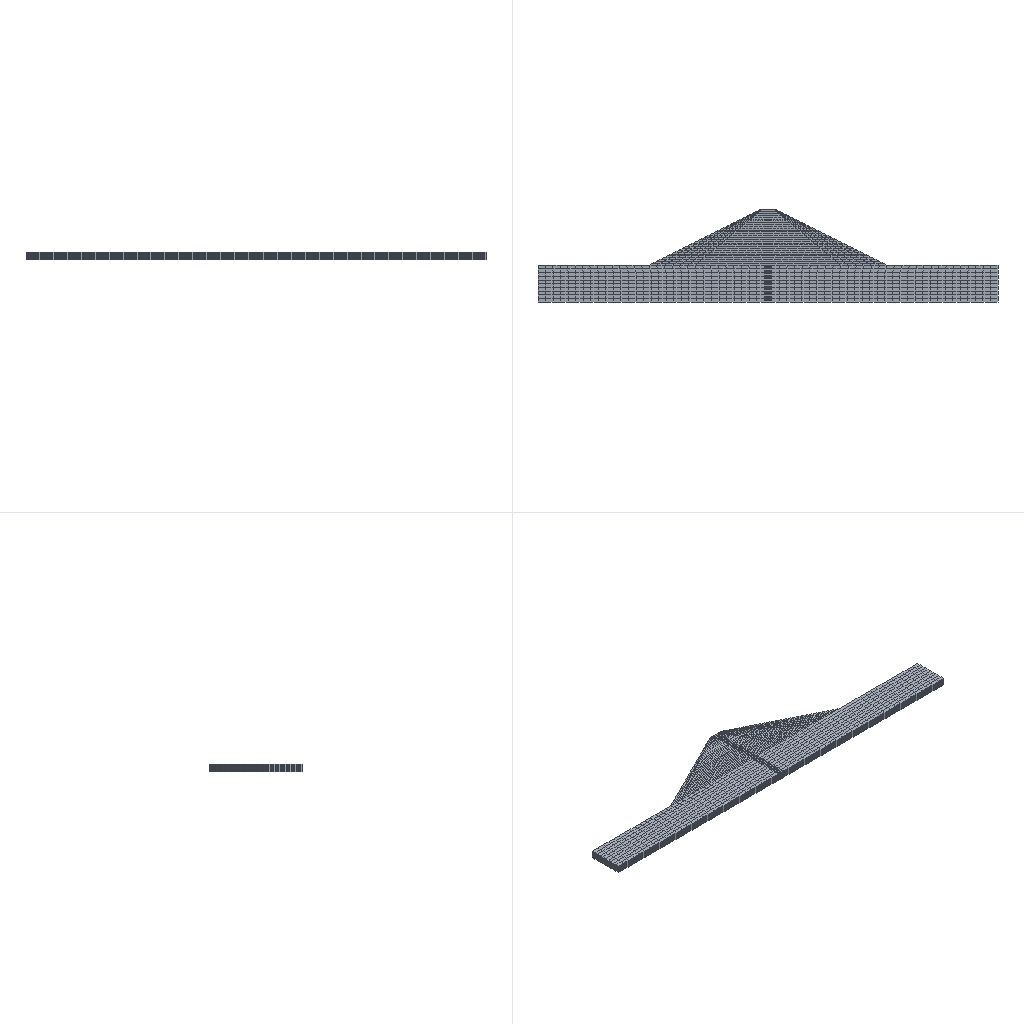Simulation study | abaqus
Set-up summary:
category,name,step,type,value,unit,region
solver,abaqus
solver,version,,,Abaqus/Standard 2020
units,not stated in the deck,,not stated
analysis,deck,,soils,soils
load_step,shenliu,shenliu,soils
load_step,requested,,,1
mesh,nodes,,,23364
mesh,elements,,,19432
element_type,C3D8P,,solid,19432
load,load commands in deck,,count,300
bc,support commands in deck,,count,311
material,BAJI,,in results
material,BATI,,in results
material,QIANG,,in results
check,setup vs results,,match,"per instance, exact: element labels, types and connectivity; labels of the nodes the elements use; coordinates of those nodes at SINGLE_PRECISION in 1 of 2 instance(s)"
Abaqus input file, long lists of numbers shortened:
*Heading
** Job name: Job-3 Model name: 3cm14mML300-OH-shenliu
** Generated by: Abaqus/CAE 2020
*Preprint, echo=NO, model=NO, history=NO, contact=NO
**
** PARTS
**
*Part, name=ba
*End Part
**
*Part, name=qiang
*End Part
**
**
** ASSEMBLY
**
*Assembly, name=Assembly
**
*Instance, name=ba-1, part=ba
*Node
      1,   62.235,         23.5,  0.9
      2,   62.235,         23.5,           0.
** (22570 more lines like these left out)
*Element, type=C3D8P
 1,     1,   169,  2647,   180,   195,  2677, 12325,  2665
 2,   169,   170,  2648,  2647,  2677,  2678, 12326, 12325
** (19078 more lines like these left out)
*Nset, nset=Set-1
     1,     2,     3,     4,     5,     6,     7,     8,     9,    10,    11,    12,    13,    14,    15,    16
    17,    18,    19,    20,    21,    22,    23,    24,    25,    26,    27,    28,    29,    30,    31,    32
** (894 more lines like these left out)
*Elset, elset=Set-1
     1,     2,     3,     4,     5,     6,     7,     8,     9,    10,    11,    12,    13,    14,    15,    16
    17,    18,    19,    20,    21,    22,    23,    24,    25,    26,    27,    28,    29,    30,    31,    32
** (748 more lines like these left out)
*Nset, nset=Set-2
    31,    32,    33,    34,    35,    36,    37,    38,    39,    40,    41,    42,    43,    44,    45,    52
    53,    54,    55,    58,    59,    62,    63,    65,    68,    69,    71,    74,    75,    77,    95,    96
** (543 more lines like these left out)
*Elset, elset=Set-2, generate
  9949,  17028,      1
** Section: bati
*Solid Section, elset=Set-1, material=bati
,
** Section: baji
*Solid Section, elset=Set-2, material=baji
,
*End Instance
**
*Instance, name=qiang-1, part=qiang
      62.235,           8.,           0.
*Node
      1,           0.,         15.5,   1.2
      2, 0.03,         15.5,   1.2
** (790 more lines like these left out)
*Element, type=C3D8P
 1,  84, 111, 110,  33,   1,   2,   3,   4
 2,  83, 112, 109,  34,  84, 111, 110,  33
** (350 more lines like these left out)
*Nset, nset=Set-1, generate
   1,  792,    1
*Elset, elset=Set-1, generate
   1,  352,    1
** Section: qiang
*Solid Section, elset=Set-1, material=qiang
,
*End Instance
**
*Nset, nset=Set-1, instance=ba-1
    31,    32,    33,    34,    35,    36,    37,    38,    39,    40,    41,    42,    43,    44,    45,    52
    53,    54,    55,    58,    59,    62,    63,    65,    68,    69,    71,    74,    75,    77,    95,    96
** (543 more lines like these left out)
*Elset, elset=Set-1, instance=ba-1, generate
  9949,  17028,      1
*Nset, nset=Set-2, instance=ba-1
   131,   132,   133,   134,   135,   136,   138,   139,   143,   144,   145,   146,   147,   148,   154,   155
   156,   158,   162,   163,   165,   166,   167,   168,  1801,  1802,  1803,  1804,  1805,  1806,  1807,  1808
** (14 more lines like these left out)
*Elset, elset=Set-2, instance=ba-1
 10961, 10962, 10963, 10964, 10965, 10966, 10967, 10968, 11085, 11086, 11087, 11088, 11321, 11322, 11323, 11324
 11325, 11326, 11327, 11328, 11525, 11526, 11527, 11528, 11529, 11530, 11531, 11532, 11533, 11534, 11535, 11536
** (11 more lines like these left out)
*Nset, nset=Set-3, instance=ba-1
    97,    98,   101,   102,   104,   106,   108,   109,   112,   115,   116,   117,   121,   122,   124,   125
   151,   152,   153,   154,   155,   156,   157,   158,   159,   160,   161,   162,   163,   164,   165,   167
** (48 more lines like these left out)
*Elset, elset=Set-3, instance=ba-1
  9963,  9964,  9979,  9980,  9995,  9996, 10011, 10012, 10041, 10042, 10043, 10044, 10073, 10074, 10075, 10076
 10105, 10106, 10107, 10108, 10137, 10138, 10139, 10140, 10148, 10156, 10185, 10186, 10187, 10188, 10301, 10302
** (43 more lines like these left out)
*Nset, nset=Set-4, instance=ba-1
     2,     3,     6,     7,    13,    15,    16,    18,    20,    22,    27,    28,    29,    30,    32,    33
    37,    39,    41,    44,    45,    46,    47,    60,    61,    62,    63,    64,    65,    67,    69,    72
** (255 more lines like these left out)
*Nset, nset=Set-4, instance=qiang-1
   9,  10,  11,  12,  17,  18,  19,  20,  21,  22,  23,  24,  26,  27,  31,  32
 145, 146, 147, 148, 149, 150, 151, 152, 153, 154, 155, 156, 157, 158, 159, 160
** (7 more lines like these left out)
*Elset, elset=Set-4, instance=ba-1
     4,     8,    12,    16,    20,    24,    28,    32,    36,    40,    44,    48,    73,    77,    81,    85
    89,    93,    97,   101,   105,   109,   113,   117,   121,   125,   129,   133,   137,   141,   145,   149
** (237 more lines like these left out)
*Elset, elset=Set-4, instance=qiang-1
  30,  33,  36,  39,  42,  45,  48,  51,  54,  57,  60,  63,  66,  69,  72,  75
  78,  81,  84,  87,  90,  93,  96,  99, 102, 105, 108, 114, 117, 120, 121, 122
** (2 more lines like these left out)
*Nset, nset=Set-6, instance=ba-1
     5,     6,    12,    19,    20,    21,    22,    24,    26,    28,    30,    31,    32,    33,    34,    35
    36,    37,    38,    39,    40,    41,    42,    43,    44,    45,    47,    52,    53,    54,    55,    56
** (599 more lines like these left out)
*Nset, nset=Set-6, instance=qiang-1
  13,  14,  15,  16,  17,  18,  19,  20,  21,  22,  23,  24,  25,  26,  27,  28
  29,  30,  31,  32, 205, 206, 207, 208, 213, 214, 215, 216, 217, 218, 219, 220
** (5 more lines like these left out)
*Elset, elset=Set-6, instance=ba-1
    33,    34,    35,    36,    65,    69,   141,   142,   143,   144,   201,   202,   203,   204,   261,   262
   263,   264,   265,   280,   295,   310,   325,   340,   355,   370,   385,   400,   415,   430,   445,   460
** (491 more lines like these left out)
*Elset, elset=Set-6, instance=qiang-1
 111, 118, 119, 120, 121, 122, 123, 126, 129, 132, 135, 138, 141, 142, 143, 144
 145, 146, 147, 148, 149, 150, 151, 152, 153, 154, 155, 156, 157, 158, 159, 160
** (2 more lines like these left out)
*Nset, nset=Set-7, instance=ba-1, generate
     1,  22572,      1
*Nset, nset=Set-7, instance=qiang-1, generate
   1,  792,    1
*Elset, elset=Set-7, instance=ba-1, generate
     1,  19080,      1
*Elset, elset=Set-7, instance=qiang-1, generate
   1,  352,    1
*Nset, nset=Set-8, instance=ba-1
    31,    32,    33,    34,    35,    36,    37,    38,    39,    40,    41,    42,    43,    44,    45,    52
    53,    54,    55,    58,    59,    62,    63,    65,    68,    69,    71,    74,    75,    77,    95,    96
** (543 more lines like these left out)
*Elset, elset=Set-8, instance=ba-1, generate
  9949,  17028,      1
*Nset, nset=Set-9, instance=ba-1
    31,    32,    33,    34,    35,    36,    37,    38,    39,    40,    41,    42,    43,    44,    45,    52
    53,    54,    55,    58,    59,    62,    63,    65,    68,    69,    71,    74,    75,    77,    95,    96
** (543 more lines like these left out)
*Elset, elset=Set-9, instance=ba-1, generate
  9949,  17028,      1
*Nset, nset=Set-10, instance=ba-1
    31,    32,    33,    34,    35,    36,    37,    38,    39,    40,    41,    42,    43,    44,    45,    52
    53,    54,    55,    58,    59,    62,    63,    65,    68,    69,    71,    74,    75,    77,    95,    96
** (543 more lines like these left out)
*Elset, elset=Set-10, instance=ba-1, generate
  9949,  17028,      1
*Nset, nset=Set-12, instance=ba-1
   19,   20,   24,   28,   40,   41,   43,   45,  247,  248,  249,  314,  352,  353,  354,  650
  651,  652,  667,  668,  669,  670,  671,  672,  673,  674,  675,  676,  677,  678,  679,  680
** (18 more lines like these left out)
*Elset, elset=Set-12, instance=ba-1
 1365, 1366, 1367, 1368, 1425, 1426, 1427, 1428, 1485, 1486, 1487, 1488, 1545, 1546, 1547, 1548
 1605, 1606, 1607, 1608, 1665, 1666, 1667, 1668, 1725, 1726, 1727, 1728, 1785, 1786, 1787, 1788
** (15 more lines like these left out)
*Nset, nset=Set-15, instance=ba-1
    31,    32,    33,    34,    35,    36,    37,    38,    39,    40,    41,    42,    43,    44,    45,    52
    53,    54,    55,    58,    59,    62,    63,    65,    68,    69,    71,    74,    75,    77,    95,    96
** (543 more lines like these left out)
*Elset, elset=Set-15, instance=ba-1, generate
  9949,  17028,      1
*Nset, nset=Set-21, instance=ba-1
    31,    32,    33,    34,    35,    36,    37,    38,    39,    40,    41,    42,    43,    44,    45,    52
    53,    54,    55,    58,    59,    62,    63,    65,    68,    69,    71,    74,    75,    77,    95,    96
** (543 more lines like these left out)
*Elset, elset=Set-21, instance=ba-1, generate
  9949,  17028,      1
*Nset, nset=Set-22, instance=ba-1
    31,    32,    33,    34,    35,    36,    37,    38,    39,    40,    41,    42,    43,    44,    45,    52
    53,    54,    55,    58,    59,    62,    63,    65,    68,    69,    71,    74,    75,    77,    95,    96
** (543 more lines like these left out)
*Elset, elset=Set-22, instance=ba-1, generate
  9949,  17028,      1
*Nset, nset=Set-23, instance=ba-1, generate
     1,  22572,      1
*Nset, nset=Set-23, instance=qiang-1, generate
   1,  792,    1
*Elset, elset=Set-23, instance=ba-1, generate
     1,  19080,      1
*Elset, elset=Set-23, instance=qiang-1, generate
   1,  352,    1
*Nset, nset=Set-33, instance=ba-1
    56,    57,    58,    59,    61,    63,    82,    83,    85,    93,    94,   150,  1009,  1038,  1039,  1040
  1041,  1042,  1043,  1044,  1045,  1046,  1047,  1048,  1049,  1050,  1051,  1052,  1053,  1054,  1055,  1056
** (20 more lines like these left out)
*Elset, elset=Set-33, instance=ba-1
  5623,  5638,  5653,  5668,  5683,  5698,  5713,  5728,  5743,  5758,  5773,  5788,  5803,  5818,  5833,  5848
  5863,  5878,  5893,  5908,  5923,  5938,  5953,  5968,  5983,  5998,  6013,  6028,  6043,  6058,  6073,  6088
** (17 more lines like these left out)
*Nset, nset=Set-34, instance=ba-1, generate
     1,  22572,      1
*Nset, nset=Set-34, instance=qiang-1, generate
   1,  792,    1
*Elset, elset=Set-34, instance=ba-1, generate
     1,  19080,      1
*Elset, elset=Set-34, instance=qiang-1, generate
   1,  352,    1
*Nset, nset=Set-35, instance=ba-1
    56,    57,    58,    59,    61,    63,    82,    83,    85,    93,    94,    97,    98,   101,   102,   104
   106,   108,   109,   112,   115,   116,   117,   121,   122,   124,   125,   143,   144,   145,   146,   147
** (86 more lines like these left out)
*Elset, elset=Set-35, instance=ba-1
  5623,  5638,  5653,  5668,  5683,  5698,  5713,  5728,  5743,  5758,  5773,  5788,  5803,  5818,  5833,  5848
  5863,  5878,  5893,  5908,  5923,  5938,  5953,  5968,  5983,  5998,  6013,  6028,  6043,  6058,  6073,  6088
** (76 more lines like these left out)
*Nset, nset=Set-36, instance=ba-1, generate
     1,  22572,      1
*Nset, nset=Set-36, instance=qiang-1, generate
   1,  792,    1
*Elset, elset=Set-36, instance=ba-1, generate
     1,  19080,      1
*Elset, elset=Set-36, instance=qiang-1, generate
   1,  352,    1
*Nset, nset=Set-39, instance=ba-1
   151,   152,   153,   154,   155,   156,   157,   158,   159,   160,   161,   162,   163,   164,   165,   167
  2188,  2189,  2190,  2198,  2199,  2200,  2201,  2202,  2203,  2204,  2205,  2206,  2207,  2208,  2209,  2210
** (37 more lines like these left out)
*Elset, elset=Set-39, instance=ba-1
 11877, 11878, 11879, 11880, 11881, 11882, 11883, 11884, 11885, 11886, 11887, 11888, 11889, 11890, 11891, 11892
 11893, 11894, 11895, 11896, 11897, 11898, 11899, 11900, 11901, 11902, 11903, 11904, 11905, 11906, 11907, 11908
** (28 more lines like these left out)
*Nset, nset=Set-41, instance=ba-1
   130,   132,   137,   138,   140,   147,   149,   153,   154,   157,   158,   159,   164,   165,   166,   167
  1866,  1867,  1868,  1869,  1870,  1871,  1872,  1873,  1874,  1875,  1876,  1877,  1878,  1879,  1880,  1881
** (68 more lines like these left out)
*Elset, elset=Set-41, instance=ba-1
 11880, 11884, 11888, 11892, 11896, 11900, 11904, 11908, 11912, 11916, 11920, 11924, 11928, 11932, 11936, 11940
 11944, 11948, 11952, 11956, 11960, 11964, 11968, 11972, 11976, 11980, 11984, 11988, 11992, 11996, 12000, 12004
** (58 more lines like these left out)
*Nset, nset=Set-44, instance=ba-1
    97,    98,   101,   102,   104,   106,   108,   109,   112,   115,   116,   117,   121,   122,   124,   125
   151,   152,   153,   154,   155,   156,   157,   158,   159,   160,   161,   162,   163,   164,   165,   167
** (48 more lines like these left out)
*Elset, elset=Set-44, instance=ba-1
  9963,  9964,  9979,  9980,  9995,  9996, 10011, 10012, 10041, 10042, 10043, 10044, 10073, 10074, 10075, 10076
 10105, 10106, 10107, 10108, 10137, 10138, 10139, 10140, 10148, 10156, 10185, 10186, 10187, 10188, 10301, 10302
** (43 more lines like these left out)
*Nset, nset=Set-45, instance=ba-1
     2,     3,    13,    15,    20,    27,    28,    32,    33,    37,    39,    41,    44,    45,    46,    60
    61,    62,    63,    64,    65,    67,    69,    72,    73,    74,    75,    76,    77,    93,   103,   104
** (239 more lines like these left out)
*Nset, nset=Set-45, instance=qiang-1
   9,  10,  11,  12,  19,  20,  23,  24,  26,  27, 145, 146, 147, 148, 149, 150
 151, 152, 153, 154, 155, 156, 157, 158, 159, 160, 161, 162, 163, 164, 165, 166
** (6 more lines like these left out)
*Elset, elset=Set-45, instance=ba-1
   556,   560,   564,   568,   572,   576,   580,   584,   588,   592,   596,   600,   604,   608,   612,   616
   620,   624,   628,   632,   636,   640,   644,   648,   652,   656,   660,   664,   668,   672,   676,   680
** (221 more lines like these left out)
*Elset, elset=Set-45, instance=qiang-1
  30,  33,  36,  39,  42,  45,  48,  51,  54,  57,  60,  63,  66,  69,  72,  75
  78,  81,  84,  87,  90,  93,  96,  99, 102, 105, 108, 142, 143, 144, 145, 146
** (2 more lines like these left out)
*Elset, elset=_Surf-26_S2, internal, instance=ba-1
  551,  552, 9353, 9354
*Surface, type=ELEMENT, name=Surf-26
_Surf-26_S2, S2
*Elset, elset=_Surf-27_S5, internal, instance=ba-1
 6489, 6490, 6491, 6492, 6549, 6550, 6551, 6552, 6609, 6610, 6611, 6612, 6669, 6670, 6671, 6672
 6729, 6730, 6731, 6732, 6789, 6790, 6791, 6792, 6849, 6850, 6851, 6852, 6909, 6910, 6911, 6912
** (5 more lines like these left out)
*Elset, elset=_Surf-27_S6, internal, instance=ba-1, generate
 5623,  6418,    15
*Elset, elset=_Surf-27_S2, internal, instance=ba-1, generate
 17029,  17136,      1
*Surface, type=ELEMENT, name=Surf-27
_Surf-27_S5, S5
_Surf-27_S6, S6
_Surf-27_S2, S2
*Elset, elset=_Surf-28_S5, internal, instance=ba-1
 6489, 6490, 6491, 6492, 6549, 6550, 6551, 6552, 6609, 6610, 6611, 6612, 6669, 6670, 6671, 6672
 6729, 6730, 6731, 6732, 6789, 6790, 6791, 6792, 6849, 6850, 6851, 6852, 6909, 6910, 6911, 6912
** (5 more lines like these left out)
*Elset, elset=_Surf-28_S6, internal, instance=ba-1, generate
 5623,  6418,    15
*Elset, elset=_Surf-28_S2, internal, instance=ba-1, generate
 17029,  17136,      1
*Surface, type=ELEMENT, name=Surf-28
_Surf-28_S5, S5
_Surf-28_S6, S6
_Surf-28_S2, S2
*Elset, elset=_ba-xia_S6, internal, instance=ba-1
 10141, 10149, 10317, 10325, 10333, 10341
*Elset, elset=_ba-xia_S3, internal, instance=ba-1, generate
 10157,  10160,      1
*Surface, type=ELEMENT, name=ba-xia
_ba-xia_S6, S6
_ba-xia_S3, S3
*Elset, elset=_ba-you_S5, internal, instance=ba-1
  8821,  8822,  8823,  8824,  8837,  8838,  8839,  8840,  8853,  8854,  8855,  8856,  8869,  8870,  8871,  8872
  8885,  8886,  8887,  8888,  8901,  8902,  8903,  8904,  8917,  8918,  8919,  8920,  8933,  8934,  8935,  8936
** (7 more lines like these left out)
*Elset, elset=_ba-you_S6, internal, instance=ba-1
 8161, 8165, 8169, 8173, 8177, 8181, 8185, 8189, 8193, 8197, 8201, 8205, 8209, 8213, 8217, 8221
 8225, 8229, 8233, 8237, 8241, 8245, 8249, 8253, 8257, 8261, 8265, 8269, 8273, 8277, 8281, 8285
** (10 more lines like these left out)
*Elset, elset=_ba-you_S3, internal, instance=ba-1
 11773, 11774, 11781, 11782
*Surface, type=ELEMENT, name=ba-you
_ba-you_S5, S5
_ba-you_S6, S6
_ba-you_S3, S3
*Elset, elset=_ba-zuo_S3, internal, instance=ba-1
     1,     2,     3,     4,    17,    18,    19,    20,    33,    34,    35,    36,   553,   554,   555,   556
   569,   570,   571,   572,   585,   586,   587,   588,   601,   602,   603,   604,   617,   618,   619,   620
** (6 more lines like these left out)
*Elset, elset=_ba-zuo_S6, internal, instance=ba-1
    49,    53,    57,    61,    65,    69,   985,   989,   993,   997,  1001,  1005,  1009,  1013,  1017,  1021
  1025,  1029,  1033,  1037,  1041,  1045,  1049,  1053,  1057,  1061,  1065,  1069,  1073,  1077,  1081,  1085
** (2 more lines like these left out)
*Elset, elset=_ba-zuo_S1, internal, instance=ba-1
  5557,  5558,  5559,  5560,  5561,  5562,  5563,  5564,  5565,  5566,  5567,  5568, 18973, 18974, 18975, 18976
 18977, 18978, 18979, 18980, 18981, 18982, 18983, 18984, 18985, 18986, 18987, 18988, 18989, 18990, 18991, 18992
** (6 more lines like these left out)
*Elset, elset=_ba-zuo_S5, internal, instance=ba-1
 10701, 10702, 10703, 10704, 10717, 10718, 10719, 10720
*Surface, type=ELEMENT, name=ba-zuo
_ba-zuo_S3, S3
_ba-zuo_S6, S6
_ba-zuo_S1, S1
_ba-zuo_S5, S5
*Elset, elset=_baxia_S2, internal, instance=ba-1
  9769,  9770,  9771,  9772,  9773,  9774,  9775,  9776,  9777,  9778,  9779,  9780, 17029, 17030, 17031, 17032
 17033, 17034, 17035, 17036, 17037, 17038, 17039, 17040, 17041, 17042, 17043, 17044, 17045, 17046, 17047, 17048
** (6 more lines like these left out)
*Elset, elset=_baxia_S6, internal, instance=ba-1
 5623, 5638, 5653, 5668, 5683, 5698, 5713, 5728, 5743, 5758, 5773, 5788, 5803, 5818, 5833, 5848
 5863, 5878, 5893, 5908, 5923, 5938, 5953, 5968, 5983, 5998, 6013, 6028, 6043, 6058, 6073, 6088
** (2 more lines like these left out)
*Elset, elset=_baxia_S5, internal, instance=ba-1
 6489, 6490, 6491, 6492, 6549, 6550, 6551, 6552, 6609, 6610, 6611, 6612, 6669, 6670, 6671, 6672
 6729, 6730, 6731, 6732, 6789, 6790, 6791, 6792, 6849, 6850, 6851, 6852, 6909, 6910, 6911, 6912
** (6 more lines like these left out)
*Surface, type=ELEMENT, name=baxia
_baxia_S2, S2
_baxia_S6, S6
_baxia_S5, S5
*Elset, elset=_fdown_S2, internal, instance=ba-1
  9769,  9770,  9771,  9772,  9773,  9774,  9775,  9776,  9777,  9778,  9779,  9780, 17029, 17030, 17031, 17032
 17033, 17034, 17035, 17036, 17037, 17038, 17039, 17040, 17041, 17042, 17043, 17044, 17045, 17046, 17047, 17048
** (6 more lines like these left out)
*Elset, elset=_fdown_S6, internal, instance=ba-1
 5623, 5638, 5653, 5668, 5683, 5698, 5713, 5728, 5743, 5758, 5773, 5788, 5803, 5818, 5833, 5848
 5863, 5878, 5893, 5908, 5923, 5938, 5953, 5968, 5983, 5998, 6013, 6028, 6043, 6058, 6073, 6088
** (2 more lines like these left out)
*Elset, elset=_fdown_S5, internal, instance=ba-1
 6489, 6490, 6491, 6492, 6549, 6550, 6551, 6552, 6609, 6610, 6611, 6612, 6669, 6670, 6671, 6672
 6729, 6730, 6731, 6732, 6789, 6790, 6791, 6792, 6849, 6850, 6851, 6852, 6909, 6910, 6911, 6912
** (6 more lines like these left out)
*Surface, type=ELEMENT, name=fdown
_fdown_S2, S2
_fdown_S6, S6
_fdown_S5, S5
*Elset, elset=_m_Surf-14_S3, internal, instance=ba-1
     1,     2,     3,     4,    17,    18,    19,    20,    33,    34,    35,    36,   553,   554,   555,   556
   569,   570,   571,   572,   585,   586,   587,   588,   601,   602,   603,   604,   617,   618,   619,   620
** (6 more lines like these left out)
*Elset, elset=_m_Surf-14_S6, internal, instance=ba-1
    49,    53,    57,    61,    65,    69,   985,   989,   993,   997,  1001,  1005,  1009,  1013,  1017,  1021
  1025,  1029,  1033,  1037,  1041,  1045,  1049,  1053,  1057,  1061,  1065,  1069,  1073,  1077,  1081,  1085
** (2 more lines like these left out)
*Elset, elset=_m_Surf-14_S1, internal, instance=ba-1
  5557,  5558,  5559,  5560,  5561,  5562,  5563,  5564,  5565,  5566,  5567,  5568, 18973, 18974, 18975, 18976
 18977, 18978, 18979, 18980, 18981, 18982, 18983, 18984, 18985, 18986, 18987, 18988, 18989, 18990, 18991, 18992
** (6 more lines like these left out)
*Elset, elset=_m_Surf-14_S5, internal, instance=ba-1
 10701, 10702, 10703, 10704, 10717, 10718, 10719, 10720
*Surface, type=ELEMENT, name=m_Surf-14
_m_Surf-14_S3, S3
_m_Surf-14_S6, S6
_m_Surf-14_S1, S1
_m_Surf-14_S5, S5
*Elset, elset=_m_Surf-16_S5, internal, instance=ba-1
  8821,  8822,  8823,  8824,  8837,  8838,  8839,  8840,  8853,  8854,  8855,  8856,  8869,  8870,  8871,  8872
  8885,  8886,  8887,  8888,  8901,  8902,  8903,  8904,  8917,  8918,  8919,  8920,  8933,  8934,  8935,  8936
** (7 more lines like these left out)
*Elset, elset=_m_Surf-16_S6, internal, instance=ba-1
 8161, 8165, 8169, 8173, 8177, 8181, 8185, 8189, 8193, 8197, 8201, 8205, 8209, 8213, 8217, 8221
 8225, 8229, 8233, 8237, 8241, 8245, 8249, 8253, 8257, 8261, 8265, 8269, 8273, 8277, 8281, 8285
** (10 more lines like these left out)
*Elset, elset=_m_Surf-16_S3, internal, instance=ba-1
 11773, 11774, 11781, 11782
*Surface, type=ELEMENT, name=m_Surf-16
_m_Surf-16_S5, S5
_m_Surf-16_S6, S6
_m_Surf-16_S3, S3
*Elset, elset=_m_Surf-18_S6, internal, instance=ba-1
 10141, 10149, 10317, 10325, 10333, 10341
*Elset, elset=_m_Surf-18_S3, internal, instance=ba-1, generate
 10157,  10160,      1
*Surface, type=ELEMENT, name=m_Surf-18
_m_Surf-18_S6, S6
_m_Surf-18_S3, S3
*Elset, elset=_qiang-xia_S6, internal, instance=qiang-1, generate
 331,  351,    2
*Surface, type=ELEMENT, name=qiang-xia
_qiang-xia_S6, S6
*Elset, elset=_qiang-you_S5, internal, instance=qiang-1
  28,  29,  30,  31,  32,  33,  34,  35,  36,  37,  38,  39,  40,  41,  42,  43
  44,  45,  46,  47,  48,  49,  50,  51,  52,  53,  54,  55,  56,  57,  58,  59
** (4 more lines like these left out)
*Elset, elset=_qiang-you_S4, internal, instance=qiang-1
   1,   2,   3,   4,   5,   6,   7,   8,   9,  10,  11,  12,  13,  14,  15,  16
  17,  18,  19,  20,  21,  22,  23,  24,  25,  26,  27, 109, 110, 111, 142, 143
** (12 more lines like these left out)
*Elset, elset=_qiang-you_S6, internal, instance=qiang-1, generate
 121,  141,    1
*Elset, elset=_qiang-you_S3, internal, instance=qiang-1, generate
 345,  352,    1
*Elset, elset=_qiang-you_S1, internal, instance=qiang-1, generate
 331,  344,    1
*Surface, type=ELEMENT, name=qiang-you
_qiang-you_S5, S5
_qiang-you_S4, S4
_qiang-you_S6, S6
_qiang-you_S3, S3
_qiang-you_S1, S1
*Elset, elset=_qiang-zuo_S3, internal, instance=qiang-1
  28,  29,  30,  31,  32,  33,  34,  35,  36,  37,  38,  39,  40,  41,  42,  43
  44,  45,  46,  47,  48,  49,  50,  51,  52,  53,  54,  55,  56,  57,  58,  59
** (4 more lines like these left out)
*Elset, elset=_qiang-zuo_S4, internal, instance=qiang-1, generate
 121,  141,    1
*Elset, elset=_qiang-zuo_S6, internal, instance=qiang-1
   1,   2,   3,   4,   5,   6,   7,   8,   9,  10,  11,  12,  13,  14,  15,  16
  17,  18,  19,  20,  21,  22,  23,  24,  25,  26,  27, 109, 110, 111, 142, 143
** (12 more lines like these left out)
*Elset, elset=_qiang-zuo_S2, internal, instance=qiang-1, generate
 331,  344,    1
*Elset, elset=_qiang-zuo_S5, internal, instance=qiang-1, generate
 345,  352,    1
*Surface, type=ELEMENT, name=qiang-zuo
_qiang-zuo_S3, S3
_qiang-zuo_S4, S4
_qiang-zuo_S6, S6
_qiang-zuo_S2, S2
_qiang-zuo_S5, S5
*Elset, elset=_qiangdi_S2, internal, instance=qiang-1
 111, 118, 119, 120
*Elset, elset=_qiangdi_S5, internal, instance=qiang-1, generate
 123,  141,    3
*Surface, type=ELEMENT, name=qiangdi
_qiangdi_S2, S2
_qiangdi_S5, S5
*Elset, elset=_s_Surf-14_S3, internal, instance=qiang-1
  28,  29,  30,  31,  32,  33,  34,  35,  36,  37,  38,  39,  40,  41,  42,  43
  44,  45,  46,  47,  48,  49,  50,  51,  52,  53,  54,  55,  56,  57,  58,  59
** (4 more lines like these left out)
*Elset, elset=_s_Surf-14_S4, internal, instance=qiang-1, generate
 121,  141,    1
*Elset, elset=_s_Surf-14_S6, internal, instance=qiang-1
   1,   2,   3,   4,   5,   6,   7,   8,   9,  10,  11,  12,  13,  14,  15,  16
  17,  18,  19,  20,  21,  22,  23,  24,  25,  26,  27, 109, 110, 111, 142, 143
** (12 more lines like these left out)
*Elset, elset=_s_Surf-14_S2, internal, instance=qiang-1, generate
 331,  344,    1
*Elset, elset=_s_Surf-14_S5, internal, instance=qiang-1, generate
 345,  352,    1
*Surface, type=ELEMENT, name=s_Surf-14
_s_Surf-14_S3, S3
_s_Surf-14_S4, S4
_s_Surf-14_S6, S6
_s_Surf-14_S2, S2
_s_Surf-14_S5, S5
*Elset, elset=_s_Surf-16_S5, internal, instance=qiang-1
  28,  29,  30,  31,  32,  33,  34,  35,  36,  37,  38,  39,  40,  41,  42,  43
  44,  45,  46,  47,  48,  49,  50,  51,  52,  53,  54,  55,  56,  57,  58,  59
** (4 more lines like these left out)
*Elset, elset=_s_Surf-16_S4, internal, instance=qiang-1
   1,   2,   3,   4,   5,   6,   7,   8,   9,  10,  11,  12,  13,  14,  15,  16
  17,  18,  19,  20,  21,  22,  23,  24,  25,  26,  27, 109, 110, 111, 142, 143
** (12 more lines like these left out)
*Elset, elset=_s_Surf-16_S6, internal, instance=qiang-1, generate
 121,  141,    1
*Elset, elset=_s_Surf-16_S3, internal, instance=qiang-1, generate
 345,  352,    1
*Elset, elset=_s_Surf-16_S1, internal, instance=qiang-1, generate
 331,  344,    1
*Surface, type=ELEMENT, name=s_Surf-16
_s_Surf-16_S5, S5
_s_Surf-16_S4, S4
_s_Surf-16_S6, S6
_s_Surf-16_S3, S3
_s_Surf-16_S1, S1
*Elset, elset=_s_Surf-18_S6, internal, instance=qiang-1, generate
 331,  351,    2
*Surface, type=ELEMENT, name=s_Surf-18
_s_Surf-18_S6, S6
*Nset, nset=Set-12_PP_, internal, instance=ba-1
   19,   20,   24,   28,   40,   41,   43,   45,  247,  248,  249,  314,  352,  353,  354,  650
  651,  652,  667,  668,  669,  670,  671,  672,  673,  674,  675,  676,  677,  678,  679,  680
** (18 more lines like these left out)
*End Assembly
**
** MATERIALS
**
*Material, name=baji
*Density
2200.,
*Elastic
 2e+08, 0.29
*Gap Flow
 0.0001,
*Permeability, specific=1000.
 1e-07, 1.5
*Material, name=bati
*Density
1930.,
*Elastic
 1e+08, 0.29
*Gap Flow
 0.0001,
*Permeability, specific=1000.
 5e-07, 1.5
*Permeability, Type=SATURATION
     1e-05, 0.02154
    0.0001, 0.04642
     0.001,       0.1
 0.07244,  0.4169
  0.9703,      0.99
        1.,        1.
*Sorption
-200000., 0.02154
-150000., 0.04642
-100000.,       0.1
 -50000.,  0.4169
 -20000.,      0.99
      0.,        1.
*Material, name=qiang
*Density
300.,
*Elastic
 1.00176e+08, 0.272
*Gap Flow
 0.0001,
*Permeability, specific=1000.
 1e-10, 1.5
**
** INTERACTION PROPERTIES
**
*Surface Interaction, name=IntProp-1
1.,
*Friction, slip tolerance=0.005
 0.1,
*Surface Behavior, penalty
**
** BOUNDARY CONDITIONS
**
** Name: x Type: Displacement/Rotation
*Boundary
Set-2, 1, 1
** PREDEFINED FIELDS
**
** Name: Predefined Field-1   Type: Saturation
*Initial Conditions, type=SATURATION
Set-7, 1.
** Name: Predefined Field-2   Type: Void ratio
*Initial Conditions, TYPE=RATIO
Set-7, 0.8
**
** INTERACTIONS
**
** Interaction: Int-4
*Contact
*Contact Inclusions, ALL EXTERIOR
*Contact Property Assignment
 ,  , IntProp-1
** ----------------------------------------------------------------
**
** STEP: shenliu
**
*Step, name=shenliu, nlgeom=NO, inc=1000
*Soils, utol=1.0, creep=none, stabilize=0.0002, allsdtol=0, continue=NO
0.001, 1., 1e-10, 1.,
*sflow
fdown,qd,0.1
**
** BOUNDARY CONDITIONS
**
** Name: BC-4 Type: 对称/反对称/完全固定
*Boundary
Set-44, ENCASTRE
** Name: BC-5 Type: 位移/转角
*Boundary
Set-45, 3, 3
** Name: shenliu Type: Pore pressure Using Analytical Field: shenliu135
*Boundary
ba-1.19, 8, 8, -0.
ba-1.20, 8, 8, -0.
ba-1.24, 8, 8, -0.
ba-1.28, 8, 8, -0.
ba-1.40, 8, 8, -135000.
ba-1.41, 8, 8, -135000.
ba-1.43, 8, 8, -135000.
ba-1.45, 8, 8, -135000.
ba-1.247, 8, 8, -0.
ba-1.248, 8, 8, -0.
ba-1.249, 8, 8, -0.
ba-1.314, 8, 8, -0.
ba-1.352, 8, 8, -0.
ba-1.353, 8, 8, -0.
ba-1.354, 8, 8, -0.
ba-1.650, 8, 8, -135000.
ba-1.651, 8, 8, -135000.
ba-1.652, 8, 8, -135000.
ba-1.667, 8, 8, -5000.
ba-1.668, 8, 8, -10000.
ba-1.669, 8, 8, -15000.
ba-1.670, 8, 8, -20000.
ba-1.671, 8, 8, -25000.
ba-1.672, 8, 8, -30000.
ba-1.673, 8, 8, -35000.
ba-1.674, 8, 8, -40000.
ba-1.675, 8, 8, -45000.
ba-1.676, 8, 8, -50000.
ba-1.677, 8, 8, -55000.
ba-1.678, 8, 8, -60000.
ba-1.679, 8, 8, -65000.
ba-1.680, 8, 8, -70000.
ba-1.681, 8, 8, -75000.
ba-1.682, 8, 8, -80000.
ba-1.683, 8, 8, -85000.
ba-1.684, 8, 8, -90000.
ba-1.685, 8, 8, -95000.
ba-1.686, 8, 8, -100000.
ba-1.687, 8, 8, -105000.
ba-1.688, 8, 8, -110000.
** (268 more lines like these left out)
**
** LOADS
**
** Name: Load-3   Type: Pressure
*Dsload
Surf-26, P, 500000.
** Name: Load-4   Type: Gravity
*Dload
, GRAV, 9.8, 0., -1., 0.
**
** CONTROLS
**
*Controls, reset
*Controls, parameters=time incrementation
, , , , , , , 20, , ,
**
** OUTPUT REQUESTS
**
*Restart, write, frequency=0
**
** FIELD OUTPUT: F-Output-2
**
*Output, field
*Node Output
POR, RF, U
*Element Output, directions=YES
E, MISES, PEMAG, S, SAT, VOIDR
*Contact Output
CSTRESS,
**
** HISTORY OUTPUT: H-Output-3
**
*Output, history
*Energy Output
ALLAE,
*End Step
Results summary:
result,step,,completed,increments=17 time=1.0/1.0
result,analysis,,,soils
result,last_loadstep,,,1
result,primary field,,,"U, POR"
result,reaction total,,FX,-0.000355,model units
result,reaction total,,FY,78554287.138,model units
result,reaction total,,FZ,-0.01185,model units